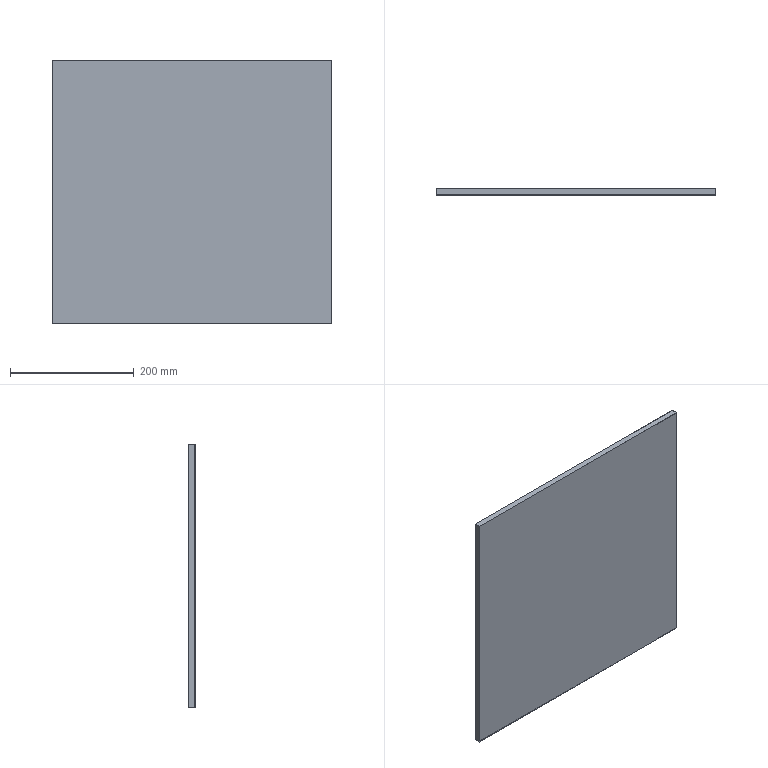Part | STEP file | Chassis side seal plate A_RR | 1 solid | 11 faces | box 452 x 10 x 427 mm | volume 208790 mm3 | plane 11
STEP:
#1=CARTESIAN_POINT('',(0.,0.,0.));
#2=DIRECTION('',(0.,0.,1.));
#3=DIRECTION('',(1.,0.,0.));
#4=AXIS2_PLACEMENT_3D('',#1,#2,#3);
#5=CARTESIAN_POINT('',(226.,0.,213.5));
#6=VERTEX_POINT('',#5);
#7=CARTESIAN_POINT('',(226.,0.,-213.5));
#8=VERTEX_POINT('',#7);
#9=CARTESIAN_POINT('',(226.,0.,0.));
#10=DIRECTION('',(0.,0.,-1.));
#11=VECTOR('',#10,1.);
#12=LINE('',#9,#11);
#13=CARTESIAN_POINT('',(0.,0.,0.));
#14=DIRECTION('',(0.,1.,0.));
#15=DIRECTION('',(0.,0.,1.));
#16=AXIS2_PLACEMENT_3D('',#13,#14,#15);
#17=PLANE('',#16);
#18=CARTESIAN_POINT('',(0.,226.));
#19=DIRECTION('',(-1.,0.));
#20=VECTOR('',#19,1.);
#21=LINE('',#18,#20);
#22=(GEOMETRIC_REPRESENTATION_CONTEXT(2)PARAMETRIC_REPRESENTATION_CONTEXT()REPRESENTATION_CONTEXT('',''));
#23=DEFINITIONAL_REPRESENTATION('',(#21),#22);
#24=PCURVE('',#17,#23);
#25=CARTESIAN_POINT('',(226.,0.,213.5));
#26=DIRECTION('',(1.,0.,0.));
#27=DIRECTION('',(0.,0.,-1.));
#28=AXIS2_PLACEMENT_3D('',#25,#26,#27);
#29=PLANE('',#28);
#30=CARTESIAN_POINT('',(213.5,0.));
#31=DIRECTION('',(1.,0.));
#32=VECTOR('',#31,1.);
#33=LINE('',#30,#32);
#34=(GEOMETRIC_REPRESENTATION_CONTEXT(2)PARAMETRIC_REPRESENTATION_CONTEXT()REPRESENTATION_CONTEXT('',''));
#35=DEFINITIONAL_REPRESENTATION('',(#33),#34);
#36=PCURVE('',#29,#35);
#37=SURFACE_CURVE('',#12,(#24,#36),.PCURVE_S1.);
#38=EDGE_CURVE('',#6,#8,#37,.T.);
#39=ORIENTED_EDGE('',*,*,#38,.F.);
#40=CARTESIAN_POINT('',(-226.,0.,213.5));
#41=VERTEX_POINT('',#40);
#42=CARTESIAN_POINT('',(0.,0.,213.5));
#43=DIRECTION('',(1.,0.,0.));
#44=VECTOR('',#43,1.);
#45=LINE('',#42,#44);
#46=CARTESIAN_POINT('',(213.5,0.));
#47=DIRECTION('',(0.,1.));
#48=VECTOR('',#47,1.);
#49=LINE('',#46,#48);
#50=(GEOMETRIC_REPRESENTATION_CONTEXT(2)PARAMETRIC_REPRESENTATION_CONTEXT()REPRESENTATION_CONTEXT('',''));
#51=DEFINITIONAL_REPRESENTATION('',(#49),#50);
#52=PCURVE('',#17,#51);
#53=CARTESIAN_POINT('',(-226.,0.,213.5));
#54=DIRECTION('',(0.,0.,1.));
#55=DIRECTION('',(1.,0.,0.));
#56=AXIS2_PLACEMENT_3D('',#53,#54,#55);
#57=PLANE('',#56);
#58=CARTESIAN_POINT('',(226.,0.));
#59=DIRECTION('',(1.,0.));
#60=VECTOR('',#59,1.);
#61=LINE('',#58,#60);
#62=(GEOMETRIC_REPRESENTATION_CONTEXT(2)PARAMETRIC_REPRESENTATION_CONTEXT()REPRESENTATION_CONTEXT('',''));
#63=DEFINITIONAL_REPRESENTATION('',(#61),#62);
#64=PCURVE('',#57,#63);
#65=SURFACE_CURVE('',#45,(#52,#64),.PCURVE_S1.);
#66=EDGE_CURVE('',#41,#6,#65,.T.);
#67=ORIENTED_EDGE('',*,*,#66,.F.);
#68=CARTESIAN_POINT('',(-226.,0.,-213.5));
#69=VERTEX_POINT('',#68);
#70=CARTESIAN_POINT('',(-226.,0.,0.));
#71=DIRECTION('',(0.,0.,1.));
#72=VECTOR('',#71,1.);
#73=LINE('',#70,#72);
#74=CARTESIAN_POINT('',(0.,-226.));
#75=DIRECTION('',(1.,0.));
#76=VECTOR('',#75,1.);
#77=LINE('',#74,#76);
#78=(GEOMETRIC_REPRESENTATION_CONTEXT(2)PARAMETRIC_REPRESENTATION_CONTEXT()REPRESENTATION_CONTEXT('',''));
#79=DEFINITIONAL_REPRESENTATION('',(#77),#78);
#80=PCURVE('',#17,#79);
#81=CARTESIAN_POINT('',(-226.,0.,-213.5));
#82=DIRECTION('',(-1.,0.,0.));
#83=DIRECTION('',(0.,0.,1.));
#84=AXIS2_PLACEMENT_3D('',#81,#82,#83);
#85=PLANE('',#84);
#86=CARTESIAN_POINT('',(213.5,0.));
#87=DIRECTION('',(1.,0.));
#88=VECTOR('',#87,1.);
#89=LINE('',#86,#88);
#90=(GEOMETRIC_REPRESENTATION_CONTEXT(2)PARAMETRIC_REPRESENTATION_CONTEXT()REPRESENTATION_CONTEXT('',''));
#91=DEFINITIONAL_REPRESENTATION('',(#89),#90);
#92=PCURVE('',#85,#91);
#93=SURFACE_CURVE('',#73,(#80,#92),.PCURVE_S1.);
#94=EDGE_CURVE('',#69,#41,#93,.T.);
#95=ORIENTED_EDGE('',*,*,#94,.F.);
#96=CARTESIAN_POINT('',(0.,0.,-213.5));
#97=DIRECTION('',(-1.,0.,0.));
#98=VECTOR('',#97,1.);
#99=LINE('',#96,#98);
#100=CARTESIAN_POINT('',(-213.5,0.));
#101=DIRECTION('',(0.,-1.));
#102=VECTOR('',#101,1.);
#103=LINE('',#100,#102);
#104=(GEOMETRIC_REPRESENTATION_CONTEXT(2)PARAMETRIC_REPRESENTATION_CONTEXT()REPRESENTATION_CONTEXT('',''));
#105=DEFINITIONAL_REPRESENTATION('',(#103),#104);
#106=PCURVE('',#17,#105);
#107=CARTESIAN_POINT('',(226.,0.,-213.5));
#108=DIRECTION('',(0.,0.,-1.));
#109=DIRECTION('',(-1.,0.,0.));
#110=AXIS2_PLACEMENT_3D('',#107,#108,#109);
#111=PLANE('',#110);
#112=CARTESIAN_POINT('',(226.,0.));
#113=DIRECTION('',(1.,0.));
#114=VECTOR('',#113,1.);
#115=LINE('',#112,#114);
#116=(GEOMETRIC_REPRESENTATION_CONTEXT(2)PARAMETRIC_REPRESENTATION_CONTEXT()REPRESENTATION_CONTEXT('',''));
#117=DEFINITIONAL_REPRESENTATION('',(#115),#116);
#118=PCURVE('',#111,#117);
#119=SURFACE_CURVE('',#99,(#106,#118),.PCURVE_S1.);
#120=EDGE_CURVE('',#8,#69,#119,.T.);
#121=ORIENTED_EDGE('',*,*,#120,.F.);
#122=EDGE_LOOP('',(#39,#67,#95,#121));
#123=FACE_BOUND('',#122,.T.);
#124=ADVANCED_FACE('',(#123),#17,.F.);
#125=CARTESIAN_POINT('',(226.,10.,-213.5));
#126=VERTEX_POINT('',#125);
#127=CARTESIAN_POINT('',(226.,0.,-213.5));
#128=DIRECTION('',(0.,-1.,0.));
#129=VECTOR('',#128,1.);
#130=LINE('',#127,#129);
#131=CARTESIAN_POINT('',(0.,0.));
#132=DIRECTION('',(0.,-1.));
#133=VECTOR('',#132,1.);
#134=LINE('',#131,#133);
#135=(GEOMETRIC_REPRESENTATION_CONTEXT(2)PARAMETRIC_REPRESENTATION_CONTEXT()REPRESENTATION_CONTEXT('',''));
#136=DEFINITIONAL_REPRESENTATION('',(#134),#135);
#137=PCURVE('',#111,#136);
#138=CARTESIAN_POINT('',(427.,0.));
#139=DIRECTION('',(0.,-1.));
#140=VECTOR('',#139,1.);
#141=LINE('',#138,#140);
#142=(GEOMETRIC_REPRESENTATION_CONTEXT(2)PARAMETRIC_REPRESENTATION_CONTEXT()REPRESENTATION_CONTEXT('',''));
#143=DEFINITIONAL_REPRESENTATION('',(#141),#142);
#144=PCURVE('',#29,#143);
#145=SURFACE_CURVE('',#130,(#137,#144),.PCURVE_S1.);
#146=EDGE_CURVE('',#126,#8,#145,.T.);
#147=ORIENTED_EDGE('',*,*,#146,.T.);
#148=ORIENTED_EDGE('',*,*,#120,.T.);
#149=CARTESIAN_POINT('',(-226.,10.,-213.5));
#150=VERTEX_POINT('',#149);
#151=CARTESIAN_POINT('',(-226.,0.,-213.5));
#152=DIRECTION('',(0.,1.,0.));
#153=VECTOR('',#152,1.);
#154=LINE('',#151,#153);
#155=CARTESIAN_POINT('',(452.,0.));
#156=DIRECTION('',(0.,1.));
#157=VECTOR('',#156,1.);
#158=LINE('',#155,#157);
#159=(GEOMETRIC_REPRESENTATION_CONTEXT(2)PARAMETRIC_REPRESENTATION_CONTEXT()REPRESENTATION_CONTEXT('',''));
#160=DEFINITIONAL_REPRESENTATION('',(#158),#159);
#161=PCURVE('',#111,#160);
#162=CARTESIAN_POINT('',(0.,0.));
#163=DIRECTION('',(0.,1.));
#164=VECTOR('',#163,1.);
#165=LINE('',#162,#164);
#166=(GEOMETRIC_REPRESENTATION_CONTEXT(2)PARAMETRIC_REPRESENTATION_CONTEXT()REPRESENTATION_CONTEXT('',''));
#167=DEFINITIONAL_REPRESENTATION('',(#165),#166);
#168=PCURVE('',#85,#167);
#169=SURFACE_CURVE('',#154,(#161,#168),.PCURVE_S1.);
#170=EDGE_CURVE('',#69,#150,#169,.T.);
#171=ORIENTED_EDGE('',*,*,#170,.T.);
#172=CARTESIAN_POINT('',(226.,10.,-213.5));
#173=DIRECTION('',(1.,0.,0.));
#174=VECTOR('',#173,1.);
#175=LINE('',#172,#174);
#176=CARTESIAN_POINT('',(0.,10.));
#177=DIRECTION('',(-1.,0.));
#178=VECTOR('',#177,1.);
#179=LINE('',#176,#178);
#180=(GEOMETRIC_REPRESENTATION_CONTEXT(2)PARAMETRIC_REPRESENTATION_CONTEXT()REPRESENTATION_CONTEXT('',''));
#181=DEFINITIONAL_REPRESENTATION('',(#179),#180);
#182=PCURVE('',#111,#181);
#183=CARTESIAN_POINT('',(0.,10.,0.));
#184=DIRECTION('',(0.,1.,0.));
#185=DIRECTION('',(0.,0.,1.));
#186=AXIS2_PLACEMENT_3D('',#183,#184,#185);
#187=PLANE('',#186);
#188=CARTESIAN_POINT('',(-213.5,226.));
#189=DIRECTION('',(0.,1.));
#190=VECTOR('',#189,1.);
#191=LINE('',#188,#190);
#192=(GEOMETRIC_REPRESENTATION_CONTEXT(2)PARAMETRIC_REPRESENTATION_CONTEXT()REPRESENTATION_CONTEXT('',''));
#193=DEFINITIONAL_REPRESENTATION('',(#191),#192);
#194=PCURVE('',#187,#193);
#195=SURFACE_CURVE('',#175,(#182,#194),.PCURVE_S1.);
#196=EDGE_CURVE('',#150,#126,#195,.T.);
#197=ORIENTED_EDGE('',*,*,#196,.T.);
#198=EDGE_LOOP('',(#147,#148,#171,#197));
#199=FACE_BOUND('',#198,.T.);
#200=ADVANCED_FACE('',(#199),#111,.T.);
#201=CARTESIAN_POINT('',(226.,10.,213.5));
#202=VERTEX_POINT('',#201);
#203=CARTESIAN_POINT('',(226.,0.,213.5));
#204=DIRECTION('',(0.,-1.,0.));
#205=VECTOR('',#204,1.);
#206=LINE('',#203,#205);
#207=CARTESIAN_POINT('',(0.,0.));
#208=DIRECTION('',(0.,-1.));
#209=VECTOR('',#208,1.);
#210=LINE('',#207,#209);
#211=(GEOMETRIC_REPRESENTATION_CONTEXT(2)PARAMETRIC_REPRESENTATION_CONTEXT()REPRESENTATION_CONTEXT('',''));
#212=DEFINITIONAL_REPRESENTATION('',(#210),#211);
#213=PCURVE('',#29,#212);
#214=CARTESIAN_POINT('',(452.,0.));
#215=DIRECTION('',(0.,-1.));
#216=VECTOR('',#215,1.);
#217=LINE('',#214,#216);
#218=(GEOMETRIC_REPRESENTATION_CONTEXT(2)PARAMETRIC_REPRESENTATION_CONTEXT()REPRESENTATION_CONTEXT('',''));
#219=DEFINITIONAL_REPRESENTATION('',(#217),#218);
#220=PCURVE('',#57,#219);
#221=SURFACE_CURVE('',#206,(#213,#220),.PCURVE_S1.);
#222=EDGE_CURVE('',#202,#6,#221,.T.);
#223=ORIENTED_EDGE('',*,*,#222,.T.);
#224=ORIENTED_EDGE('',*,*,#38,.T.);
#225=ORIENTED_EDGE('',*,*,#146,.F.);
#226=CARTESIAN_POINT('',(226.,10.,213.5));
#227=DIRECTION('',(0.,0.,1.));
#228=VECTOR('',#227,1.);
#229=LINE('',#226,#228);
#230=CARTESIAN_POINT('',(0.,10.));
#231=DIRECTION('',(-1.,0.));
#232=VECTOR('',#231,1.);
#233=LINE('',#230,#232);
#234=(GEOMETRIC_REPRESENTATION_CONTEXT(2)PARAMETRIC_REPRESENTATION_CONTEXT()REPRESENTATION_CONTEXT('',''));
#235=DEFINITIONAL_REPRESENTATION('',(#233),#234);
#236=PCURVE('',#29,#235);
#237=CARTESIAN_POINT('',(213.5,226.));
#238=DIRECTION('',(1.,0.));
#239=VECTOR('',#238,1.);
#240=LINE('',#237,#239);
#241=(GEOMETRIC_REPRESENTATION_CONTEXT(2)PARAMETRIC_REPRESENTATION_CONTEXT()REPRESENTATION_CONTEXT('',''));
#242=DEFINITIONAL_REPRESENTATION('',(#240),#241);
#243=PCURVE('',#187,#242);
#244=SURFACE_CURVE('',#229,(#236,#243),.PCURVE_S1.);
#245=EDGE_CURVE('',#126,#202,#244,.T.);
#246=ORIENTED_EDGE('',*,*,#245,.T.);
#247=EDGE_LOOP('',(#223,#224,#225,#246));
#248=FACE_BOUND('',#247,.T.);
#249=ADVANCED_FACE('',(#248),#29,.T.);
#250=CARTESIAN_POINT('',(-226.,10.,213.5));
#251=VERTEX_POINT('',#250);
#252=CARTESIAN_POINT('',(-226.,0.,213.5));
#253=DIRECTION('',(0.,-1.,0.));
#254=VECTOR('',#253,1.);
#255=LINE('',#252,#254);
#256=CARTESIAN_POINT('',(0.,0.));
#257=DIRECTION('',(0.,-1.));
#258=VECTOR('',#257,1.);
#259=LINE('',#256,#258);
#260=(GEOMETRIC_REPRESENTATION_CONTEXT(2)PARAMETRIC_REPRESENTATION_CONTEXT()REPRESENTATION_CONTEXT('',''));
#261=DEFINITIONAL_REPRESENTATION('',(#259),#260);
#262=PCURVE('',#57,#261);
#263=CARTESIAN_POINT('',(427.,0.));
#264=DIRECTION('',(0.,-1.));
#265=VECTOR('',#264,1.);
#266=LINE('',#263,#265);
#267=(GEOMETRIC_REPRESENTATION_CONTEXT(2)PARAMETRIC_REPRESENTATION_CONTEXT()REPRESENTATION_CONTEXT('',''));
#268=DEFINITIONAL_REPRESENTATION('',(#266),#267);
#269=PCURVE('',#85,#268);
#270=SURFACE_CURVE('',#255,(#262,#269),.PCURVE_S1.);
#271=EDGE_CURVE('',#251,#41,#270,.T.);
#272=ORIENTED_EDGE('',*,*,#271,.T.);
#273=ORIENTED_EDGE('',*,*,#66,.T.);
#274=ORIENTED_EDGE('',*,*,#222,.F.);
#275=CARTESIAN_POINT('',(-226.,10.,213.5));
#276=DIRECTION('',(-1.,0.,0.));
#277=VECTOR('',#276,1.);
#278=LINE('',#275,#277);
#279=CARTESIAN_POINT('',(0.,10.));
#280=DIRECTION('',(-1.,0.));
#281=VECTOR('',#280,1.);
#282=LINE('',#279,#281);
#283=(GEOMETRIC_REPRESENTATION_CONTEXT(2)PARAMETRIC_REPRESENTATION_CONTEXT()REPRESENTATION_CONTEXT('',''));
#284=DEFINITIONAL_REPRESENTATION('',(#282),#283);
#285=PCURVE('',#57,#284);
#286=CARTESIAN_POINT('',(213.5,-226.));
#287=DIRECTION('',(0.,-1.));
#288=VECTOR('',#287,1.);
#289=LINE('',#286,#288);
#290=(GEOMETRIC_REPRESENTATION_CONTEXT(2)PARAMETRIC_REPRESENTATION_CONTEXT()REPRESENTATION_CONTEXT('',''));
#291=DEFINITIONAL_REPRESENTATION('',(#289),#290);
#292=PCURVE('',#187,#291);
#293=SURFACE_CURVE('',#278,(#285,#292),.PCURVE_S1.);
#294=EDGE_CURVE('',#202,#251,#293,.T.);
#295=ORIENTED_EDGE('',*,*,#294,.T.);
#296=EDGE_LOOP('',(#272,#273,#274,#295));
#297=FACE_BOUND('',#296,.T.);
#298=ADVANCED_FACE('',(#297),#57,.T.);
#299=ORIENTED_EDGE('',*,*,#170,.F.);
#300=ORIENTED_EDGE('',*,*,#94,.T.);
#301=ORIENTED_EDGE('',*,*,#271,.F.);
#302=CARTESIAN_POINT('',(-226.,10.,-213.5));
#303=DIRECTION('',(0.,0.,-1.));
#304=VECTOR('',#303,1.);
#305=LINE('',#302,#304);
#306=CARTESIAN_POINT('',(0.,10.));
#307=DIRECTION('',(-1.,0.));
#308=VECTOR('',#307,1.);
#309=LINE('',#306,#308);
#310=(GEOMETRIC_REPRESENTATION_CONTEXT(2)PARAMETRIC_REPRESENTATION_CONTEXT()REPRESENTATION_CONTEXT('',''));
#311=DEFINITIONAL_REPRESENTATION('',(#309),#310);
#312=PCURVE('',#85,#311);
#313=CARTESIAN_POINT('',(-213.5,-226.));
#314=DIRECTION('',(-1.,0.));
#315=VECTOR('',#314,1.);
#316=LINE('',#313,#315);
#317=(GEOMETRIC_REPRESENTATION_CONTEXT(2)PARAMETRIC_REPRESENTATION_CONTEXT()REPRESENTATION_CONTEXT('',''));
#318=DEFINITIONAL_REPRESENTATION('',(#316),#317);
#319=PCURVE('',#187,#318);
#320=SURFACE_CURVE('',#305,(#312,#319),.PCURVE_S1.);
#321=EDGE_CURVE('',#251,#150,#320,.T.);
#322=ORIENTED_EDGE('',*,*,#321,.T.);
#323=EDGE_LOOP('',(#299,#300,#301,#322));
#324=FACE_BOUND('',#323,.T.);
#325=ADVANCED_FACE('',(#324),#85,.T.);
#326=CARTESIAN_POINT('',(225.,10.,212.5));
#327=VERTEX_POINT('',#326);
#328=CARTESIAN_POINT('',(-225.,10.,212.5));
#329=VERTEX_POINT('',#328);
#330=CARTESIAN_POINT('',(0.,10.,212.5));
#331=DIRECTION('',(-1.,0.,0.));
#332=VECTOR('',#331,1.);
#333=LINE('',#330,#332);
#334=CARTESIAN_POINT('',(212.5,0.));
#335=DIRECTION('',(0.,-1.));
#336=VECTOR('',#335,1.);
#337=LINE('',#334,#336);
#338=(GEOMETRIC_REPRESENTATION_CONTEXT(2)PARAMETRIC_REPRESENTATION_CONTEXT()REPRESENTATION_CONTEXT('',''));
#339=DEFINITIONAL_REPRESENTATION('',(#337),#338);
#340=PCURVE('',#187,#339);
#341=CARTESIAN_POINT('',(-226.,0.,212.5));
#342=DIRECTION('',(0.,0.,1.));
#343=DIRECTION('',(1.,0.,0.));
#344=AXIS2_PLACEMENT_3D('',#341,#342,#343);
#345=PLANE('',#344);
#346=CARTESIAN_POINT('',(226.,10.));
#347=DIRECTION('',(-1.,0.));
#348=VECTOR('',#347,1.);
#349=LINE('',#346,#348);
#350=(GEOMETRIC_REPRESENTATION_CONTEXT(2)PARAMETRIC_REPRESENTATION_CONTEXT()REPRESENTATION_CONTEXT('',''));
#351=DEFINITIONAL_REPRESENTATION('',(#349),#350);
#352=PCURVE('',#345,#351);
#353=SURFACE_CURVE('',#333,(#340,#352),.PCURVE_S1.);
#354=EDGE_CURVE('',#327,#329,#353,.T.);
#355=ORIENTED_EDGE('',*,*,#354,.T.);
#356=CARTESIAN_POINT('',(-225.,10.,-212.5));
#357=VERTEX_POINT('',#356);
#358=CARTESIAN_POINT('',(-225.,10.,0.));
#359=DIRECTION('',(0.,0.,-1.));
#360=VECTOR('',#359,1.);
#361=LINE('',#358,#360);
#362=CARTESIAN_POINT('',(0.,-225.));
#363=DIRECTION('',(-1.,0.));
#364=VECTOR('',#363,1.);
#365=LINE('',#362,#364);
#366=(GEOMETRIC_REPRESENTATION_CONTEXT(2)PARAMETRIC_REPRESENTATION_CONTEXT()REPRESENTATION_CONTEXT('',''));
#367=DEFINITIONAL_REPRESENTATION('',(#365),#366);
#368=PCURVE('',#187,#367);
#369=CARTESIAN_POINT('',(-225.,0.,-213.5));
#370=DIRECTION('',(-1.,0.,0.));
#371=DIRECTION('',(0.,0.,1.));
#372=AXIS2_PLACEMENT_3D('',#369,#370,#371);
#373=PLANE('',#372);
#374=CARTESIAN_POINT('',(213.5,10.));
#375=DIRECTION('',(-1.,0.));
#376=VECTOR('',#375,1.);
#377=LINE('',#374,#376);
#378=(GEOMETRIC_REPRESENTATION_CONTEXT(2)PARAMETRIC_REPRESENTATION_CONTEXT()REPRESENTATION_CONTEXT('',''));
#379=DEFINITIONAL_REPRESENTATION('',(#377),#378);
#380=PCURVE('',#373,#379);
#381=SURFACE_CURVE('',#361,(#368,#380),.PCURVE_S1.);
#382=EDGE_CURVE('',#329,#357,#381,.T.);
#383=ORIENTED_EDGE('',*,*,#382,.T.);
#384=CARTESIAN_POINT('',(225.,10.,-212.5));
#385=VERTEX_POINT('',#384);
#386=CARTESIAN_POINT('',(0.,10.,-212.5));
#387=DIRECTION('',(1.,0.,0.));
#388=VECTOR('',#387,1.);
#389=LINE('',#386,#388);
#390=CARTESIAN_POINT('',(-212.5,0.));
#391=DIRECTION('',(0.,1.));
#392=VECTOR('',#391,1.);
#393=LINE('',#390,#392);
#394=(GEOMETRIC_REPRESENTATION_CONTEXT(2)PARAMETRIC_REPRESENTATION_CONTEXT()REPRESENTATION_CONTEXT('',''));
#395=DEFINITIONAL_REPRESENTATION('',(#393),#394);
#396=PCURVE('',#187,#395);
#397=CARTESIAN_POINT('',(226.,0.,-212.5));
#398=DIRECTION('',(0.,0.,-1.));
#399=DIRECTION('',(-1.,0.,0.));
#400=AXIS2_PLACEMENT_3D('',#397,#398,#399);
#401=PLANE('',#400);
#402=CARTESIAN_POINT('',(226.,10.));
#403=DIRECTION('',(-1.,0.));
#404=VECTOR('',#403,1.);
#405=LINE('',#402,#404);
#406=(GEOMETRIC_REPRESENTATION_CONTEXT(2)PARAMETRIC_REPRESENTATION_CONTEXT()REPRESENTATION_CONTEXT('',''));
#407=DEFINITIONAL_REPRESENTATION('',(#405),#406);
#408=PCURVE('',#401,#407);
#409=SURFACE_CURVE('',#389,(#396,#408),.PCURVE_S1.);
#410=EDGE_CURVE('',#357,#385,#409,.T.);
#411=ORIENTED_EDGE('',*,*,#410,.T.);
#412=CARTESIAN_POINT('',(225.,10.,0.));
#413=DIRECTION('',(0.,0.,1.));
#414=VECTOR('',#413,1.);
#415=LINE('',#412,#414);
#416=CARTESIAN_POINT('',(0.,225.));
#417=DIRECTION('',(1.,0.));
#418=VECTOR('',#417,1.);
#419=LINE('',#416,#418);
#420=(GEOMETRIC_REPRESENTATION_CONTEXT(2)PARAMETRIC_REPRESENTATION_CONTEXT()REPRESENTATION_CONTEXT('',''));
#421=DEFINITIONAL_REPRESENTATION('',(#419),#420);
#422=PCURVE('',#187,#421);
#423=CARTESIAN_POINT('',(225.,0.,213.5));
#424=DIRECTION('',(1.,0.,0.));
#425=DIRECTION('',(0.,0.,-1.));
#426=AXIS2_PLACEMENT_3D('',#423,#424,#425);
#427=PLANE('',#426);
#428=CARTESIAN_POINT('',(213.5,10.));
#429=DIRECTION('',(-1.,0.));
#430=VECTOR('',#429,1.);
#431=LINE('',#428,#430);
#432=(GEOMETRIC_REPRESENTATION_CONTEXT(2)PARAMETRIC_REPRESENTATION_CONTEXT()REPRESENTATION_CONTEXT('',''));
#433=DEFINITIONAL_REPRESENTATION('',(#431),#432);
#434=PCURVE('',#427,#433);
#435=SURFACE_CURVE('',#415,(#422,#434),.PCURVE_S1.);
#436=EDGE_CURVE('',#385,#327,#435,.T.);
#437=ORIENTED_EDGE('',*,*,#436,.T.);
#438=EDGE_LOOP('',(#355,#383,#411,#437));
#439=FACE_BOUND('',#438,.T.);
#440=ORIENTED_EDGE('',*,*,#196,.F.);
#441=ORIENTED_EDGE('',*,*,#321,.F.);
#442=ORIENTED_EDGE('',*,*,#294,.F.);
#443=ORIENTED_EDGE('',*,*,#245,.F.);
#444=EDGE_LOOP('',(#440,#441,#442,#443));
#445=FACE_BOUND('',#444,.T.);
#446=ADVANCED_FACE('',(#439,#445),#187,.T.);
#447=CARTESIAN_POINT('',(-225.,1.,-212.5));
#448=VERTEX_POINT('',#447);
#449=CARTESIAN_POINT('',(-225.,1.,212.5));
#450=VERTEX_POINT('',#449);
#451=CARTESIAN_POINT('',(-225.,1.,-213.5));
#452=DIRECTION('',(0.,0.,1.));
#453=VECTOR('',#452,1.);
#454=LINE('',#451,#453);
#455=CARTESIAN_POINT('',(0.,1.));
#456=DIRECTION('',(1.,0.));
#457=VECTOR('',#456,1.);
#458=LINE('',#455,#457);
#459=(GEOMETRIC_REPRESENTATION_CONTEXT(2)PARAMETRIC_REPRESENTATION_CONTEXT()REPRESENTATION_CONTEXT('',''));
#460=DEFINITIONAL_REPRESENTATION('',(#458),#459);
#461=PCURVE('',#373,#460);
#462=CARTESIAN_POINT('',(0.,1.,0.));
#463=DIRECTION('',(0.,1.,0.));
#464=DIRECTION('',(0.,0.,1.));
#465=AXIS2_PLACEMENT_3D('',#462,#463,#464);
#466=PLANE('',#465);
#467=CARTESIAN_POINT('',(-213.5,-225.));
#468=DIRECTION('',(1.,0.));
#469=VECTOR('',#468,1.);
#470=LINE('',#467,#469);
#471=(GEOMETRIC_REPRESENTATION_CONTEXT(2)PARAMETRIC_REPRESENTATION_CONTEXT()REPRESENTATION_CONTEXT('',''));
#472=DEFINITIONAL_REPRESENTATION('',(#470),#471);
#473=PCURVE('',#466,#472);
#474=SURFACE_CURVE('',#454,(#461,#473),.PCURVE_S1.);
#475=EDGE_CURVE('',#448,#450,#474,.T.);
#476=ORIENTED_EDGE('',*,*,#475,.F.);
#477=CARTESIAN_POINT('',(-225.,0.,-212.5));
#478=DIRECTION('',(0.,-1.,0.));
#479=VECTOR('',#478,1.);
#480=LINE('',#477,#479);
#481=CARTESIAN_POINT('',(1.,0.));
#482=DIRECTION('',(0.,-1.));
#483=VECTOR('',#482,1.);
#484=LINE('',#481,#483);
#485=(GEOMETRIC_REPRESENTATION_CONTEXT(2)PARAMETRIC_REPRESENTATION_CONTEXT()REPRESENTATION_CONTEXT('',''));
#486=DEFINITIONAL_REPRESENTATION('',(#484),#485);
#487=PCURVE('',#373,#486);
#488=CARTESIAN_POINT('',(451.,0.));
#489=DIRECTION('',(0.,-1.));
#490=VECTOR('',#489,1.);
#491=LINE('',#488,#490);
#492=(GEOMETRIC_REPRESENTATION_CONTEXT(2)PARAMETRIC_REPRESENTATION_CONTEXT()REPRESENTATION_CONTEXT('',''));
#493=DEFINITIONAL_REPRESENTATION('',(#491),#492);
#494=PCURVE('',#401,#493);
#495=SURFACE_CURVE('',#480,(#487,#494),.PCURVE_S1.);
#496=EDGE_CURVE('',#357,#448,#495,.T.);
#497=ORIENTED_EDGE('',*,*,#496,.F.);
#498=ORIENTED_EDGE('',*,*,#382,.F.);
#499=CARTESIAN_POINT('',(-225.,0.,212.5));
#500=DIRECTION('',(0.,1.,0.));
#501=VECTOR('',#500,1.);
#502=LINE('',#499,#501);
#503=CARTESIAN_POINT('',(426.,0.));
#504=DIRECTION('',(0.,1.));
#505=VECTOR('',#504,1.);
#506=LINE('',#503,#505);
#507=(GEOMETRIC_REPRESENTATION_CONTEXT(2)PARAMETRIC_REPRESENTATION_CONTEXT()REPRESENTATION_CONTEXT('',''));
#508=DEFINITIONAL_REPRESENTATION('',(#506),#507);
#509=PCURVE('',#373,#508);
#510=CARTESIAN_POINT('',(1.,0.));
#511=DIRECTION('',(0.,1.));
#512=VECTOR('',#511,1.);
#513=LINE('',#510,#512);
#514=(GEOMETRIC_REPRESENTATION_CONTEXT(2)PARAMETRIC_REPRESENTATION_CONTEXT()REPRESENTATION_CONTEXT('',''));
#515=DEFINITIONAL_REPRESENTATION('',(#513),#514);
#516=PCURVE('',#345,#515);
#517=SURFACE_CURVE('',#502,(#509,#516),.PCURVE_S1.);
#518=EDGE_CURVE('',#450,#329,#517,.T.);
#519=ORIENTED_EDGE('',*,*,#518,.F.);
#520=EDGE_LOOP('',(#476,#497,#498,#519));
#521=FACE_BOUND('',#520,.T.);
#522=ADVANCED_FACE('',(#521),#373,.F.);
#523=CARTESIAN_POINT('',(225.,1.,212.5));
#524=VERTEX_POINT('',#523);
#525=CARTESIAN_POINT('',(-226.,1.,212.5));
#526=DIRECTION('',(1.,0.,0.));
#527=VECTOR('',#526,1.);
#528=LINE('',#525,#527);
#529=CARTESIAN_POINT('',(0.,1.));
#530=DIRECTION('',(1.,0.));
#531=VECTOR('',#530,1.);
#532=LINE('',#529,#531);
#533=(GEOMETRIC_REPRESENTATION_CONTEXT(2)PARAMETRIC_REPRESENTATION_CONTEXT()REPRESENTATION_CONTEXT('',''));
#534=DEFINITIONAL_REPRESENTATION('',(#532),#533);
#535=PCURVE('',#345,#534);
#536=CARTESIAN_POINT('',(212.5,-226.));
#537=DIRECTION('',(0.,1.));
#538=VECTOR('',#537,1.);
#539=LINE('',#536,#538);
#540=(GEOMETRIC_REPRESENTATION_CONTEXT(2)PARAMETRIC_REPRESENTATION_CONTEXT()REPRESENTATION_CONTEXT('',''));
#541=DEFINITIONAL_REPRESENTATION('',(#539),#540);
#542=PCURVE('',#466,#541);
#543=SURFACE_CURVE('',#528,(#535,#542),.PCURVE_S1.);
#544=EDGE_CURVE('',#450,#524,#543,.T.);
#545=ORIENTED_EDGE('',*,*,#544,.F.);
#546=ORIENTED_EDGE('',*,*,#518,.T.);
#547=ORIENTED_EDGE('',*,*,#354,.F.);
#548=CARTESIAN_POINT('',(225.,0.,212.5));
#549=DIRECTION('',(0.,1.,0.));
#550=VECTOR('',#549,1.);
#551=LINE('',#548,#550);
#552=CARTESIAN_POINT('',(451.,0.));
#553=DIRECTION('',(0.,1.));
#554=VECTOR('',#553,1.);
#555=LINE('',#552,#554);
#556=(GEOMETRIC_REPRESENTATION_CONTEXT(2)PARAMETRIC_REPRESENTATION_CONTEXT()REPRESENTATION_CONTEXT('',''));
#557=DEFINITIONAL_REPRESENTATION('',(#555),#556);
#558=PCURVE('',#345,#557);
#559=CARTESIAN_POINT('',(1.,0.));
#560=DIRECTION('',(0.,1.));
#561=VECTOR('',#560,1.);
#562=LINE('',#559,#561);
#563=(GEOMETRIC_REPRESENTATION_CONTEXT(2)PARAMETRIC_REPRESENTATION_CONTEXT()REPRESENTATION_CONTEXT('',''));
#564=DEFINITIONAL_REPRESENTATION('',(#562),#563);
#565=PCURVE('',#427,#564);
#566=SURFACE_CURVE('',#551,(#558,#565),.PCURVE_S1.);
#567=EDGE_CURVE('',#524,#327,#566,.T.);
#568=ORIENTED_EDGE('',*,*,#567,.F.);
#569=EDGE_LOOP('',(#545,#546,#547,#568));
#570=FACE_BOUND('',#569,.T.);
#571=ADVANCED_FACE('',(#570),#345,.F.);
#572=CARTESIAN_POINT('',(225.,1.,-212.5));
#573=VERTEX_POINT('',#572);
#574=CARTESIAN_POINT('',(225.,1.,213.5));
#575=DIRECTION('',(0.,0.,-1.));
#576=VECTOR('',#575,1.);
#577=LINE('',#574,#576);
#578=CARTESIAN_POINT('',(0.,1.));
#579=DIRECTION('',(1.,0.));
#580=VECTOR('',#579,1.);
#581=LINE('',#578,#580);
#582=(GEOMETRIC_REPRESENTATION_CONTEXT(2)PARAMETRIC_REPRESENTATION_CONTEXT()REPRESENTATION_CONTEXT('',''));
#583=DEFINITIONAL_REPRESENTATION('',(#581),#582);
#584=PCURVE('',#427,#583);
#585=CARTESIAN_POINT('',(213.5,225.));
#586=DIRECTION('',(-1.,0.));
#587=VECTOR('',#586,1.);
#588=LINE('',#585,#587);
#589=(GEOMETRIC_REPRESENTATION_CONTEXT(2)PARAMETRIC_REPRESENTATION_CONTEXT()REPRESENTATION_CONTEXT('',''));
#590=DEFINITIONAL_REPRESENTATION('',(#588),#589);
#591=PCURVE('',#466,#590);
#592=SURFACE_CURVE('',#577,(#584,#591),.PCURVE_S1.);
#593=EDGE_CURVE('',#524,#573,#592,.T.);
#594=ORIENTED_EDGE('',*,*,#593,.F.);
#595=ORIENTED_EDGE('',*,*,#567,.T.);
#596=ORIENTED_EDGE('',*,*,#436,.F.);
#597=CARTESIAN_POINT('',(225.,0.,-212.5));
#598=DIRECTION('',(0.,1.,0.));
#599=VECTOR('',#598,1.);
#600=LINE('',#597,#599);
#601=CARTESIAN_POINT('',(426.,0.));
#602=DIRECTION('',(0.,1.));
#603=VECTOR('',#602,1.);
#604=LINE('',#601,#603);
#605=(GEOMETRIC_REPRESENTATION_CONTEXT(2)PARAMETRIC_REPRESENTATION_CONTEXT()REPRESENTATION_CONTEXT('',''));
#606=DEFINITIONAL_REPRESENTATION('',(#604),#605);
#607=PCURVE('',#427,#606);
#608=CARTESIAN_POINT('',(1.,0.));
#609=DIRECTION('',(0.,1.));
#610=VECTOR('',#609,1.);
#611=LINE('',#608,#610);
#612=(GEOMETRIC_REPRESENTATION_CONTEXT(2)PARAMETRIC_REPRESENTATION_CONTEXT()REPRESENTATION_CONTEXT('',''));
#613=DEFINITIONAL_REPRESENTATION('',(#611),#612);
#614=PCURVE('',#401,#613);
#615=SURFACE_CURVE('',#600,(#607,#614),.PCURVE_S1.);
#616=EDGE_CURVE('',#573,#385,#615,.T.);
#617=ORIENTED_EDGE('',*,*,#616,.F.);
#618=EDGE_LOOP('',(#594,#595,#596,#617));
#619=FACE_BOUND('',#618,.T.);
#620=ADVANCED_FACE('',(#619),#427,.F.);
#621=CARTESIAN_POINT('',(226.,1.,-212.5));
#622=DIRECTION('',(-1.,0.,0.));
#623=VECTOR('',#622,1.);
#624=LINE('',#621,#623);
#625=CARTESIAN_POINT('',(0.,1.));
#626=DIRECTION('',(1.,0.));
#627=VECTOR('',#626,1.);
#628=LINE('',#625,#627);
#629=(GEOMETRIC_REPRESENTATION_CONTEXT(2)PARAMETRIC_REPRESENTATION_CONTEXT()REPRESENTATION_CONTEXT('',''));
#630=DEFINITIONAL_REPRESENTATION('',(#628),#629);
#631=PCURVE('',#401,#630);
#632=CARTESIAN_POINT('',(-212.5,226.));
#633=DIRECTION('',(0.,-1.));
#634=VECTOR('',#633,1.);
#635=LINE('',#632,#634);
#636=(GEOMETRIC_REPRESENTATION_CONTEXT(2)PARAMETRIC_REPRESENTATION_CONTEXT()REPRESENTATION_CONTEXT('',''));
#637=DEFINITIONAL_REPRESENTATION('',(#635),#636);
#638=PCURVE('',#466,#637);
#639=SURFACE_CURVE('',#624,(#631,#638),.PCURVE_S1.);
#640=EDGE_CURVE('',#573,#448,#639,.T.);
#641=ORIENTED_EDGE('',*,*,#640,.F.);
#642=ORIENTED_EDGE('',*,*,#616,.T.);
#643=ORIENTED_EDGE('',*,*,#410,.F.);
#644=ORIENTED_EDGE('',*,*,#496,.T.);
#645=EDGE_LOOP('',(#641,#642,#643,#644));
#646=FACE_BOUND('',#645,.T.);
#647=ADVANCED_FACE('',(#646),#401,.F.);
#648=ORIENTED_EDGE('',*,*,#640,.T.);
#649=ORIENTED_EDGE('',*,*,#475,.T.);
#650=ORIENTED_EDGE('',*,*,#544,.T.);
#651=ORIENTED_EDGE('',*,*,#593,.T.);
#652=EDGE_LOOP('',(#648,#649,#650,#651));
#653=FACE_BOUND('',#652,.T.);
#654=ADVANCED_FACE('',(#653),#466,.T.);
#655=CLOSED_SHELL('',(#124,#200,#249,#298,#325,#446,#522,#571,#620,#647,#654));
#656=MANIFOLD_SOLID_BREP('',#655);
#657=(LENGTH_UNIT()NAMED_UNIT(*)SI_UNIT(.MILLI.,.METRE.));
#658=UNCERTAINTY_MEASURE_WITH_UNIT(LENGTH_MEASURE(0.0000001),#657,'','');
#659=(NAMED_UNIT(*)PLANE_ANGLE_UNIT()SI_UNIT($,.RADIAN.));
#660=(NAMED_UNIT(*)SI_UNIT($,.STERADIAN.)SOLID_ANGLE_UNIT());
#661=(GEOMETRIC_REPRESENTATION_CONTEXT(3)GLOBAL_UNCERTAINTY_ASSIGNED_CONTEXT((#658))GLOBAL_UNIT_ASSIGNED_CONTEXT((#657,#659,#660))REPRESENTATION_CONTEXT('',''));
#662=ADVANCED_BREP_SHAPE_REPRESENTATION('',(#4,#656),#661);